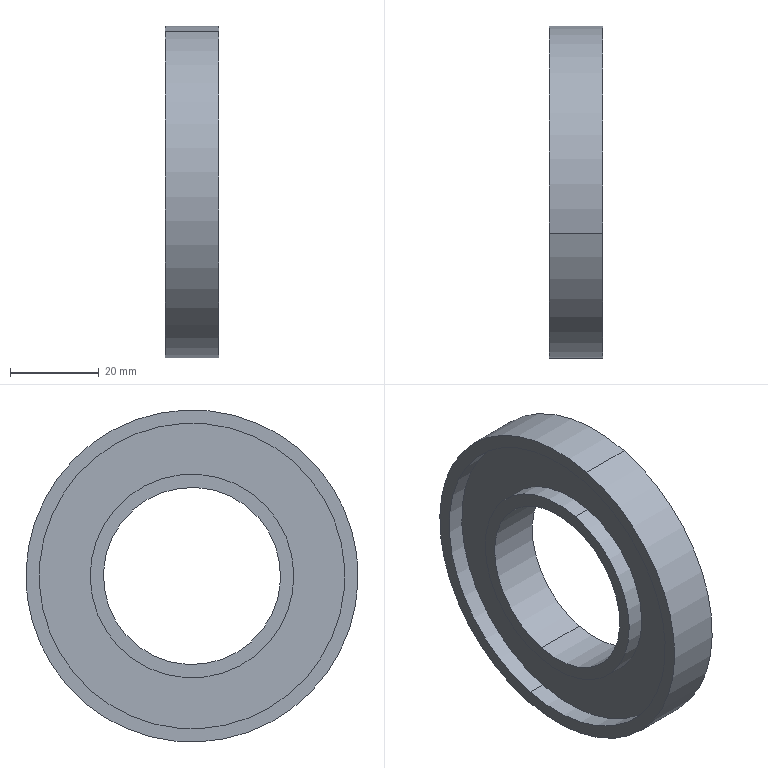Part | NX | features BREP 1 | 1 solid | 18 faces | box 12 x 75 x 75 mm | volume 21316 mm3 | cylinder 12 | plane 6 | commonest cylinder face diameters 46 x4 69 x4 40 x2 75 x2
STEP:
#1=CARTESIAN_POINT('',(691.455,5.743,-22.271));
#2=VERTEX_POINT('',#1);
#3=CARTESIAN_POINT('',(691.455,-5.743,22.271));
#4=VERTEX_POINT('',#3);
#5=CARTESIAN_POINT('',(691.455,0.,0.));
#6=DIRECTION('',(-1.,0.,0.));
#7=DIRECTION('',(0.,-0.2497,0.9683));
#8=AXIS2_PLACEMENT_3D('',#5,#6,#7);
#9=CIRCLE('',#8,23.);
#10=EDGE_CURVE('',#2,#4,#9,.T.);
#11=ORIENTED_EDGE('',*,*,#10,.T.);
#12=CARTESIAN_POINT('',(687.455,-5.743,22.271));
#13=VERTEX_POINT('',#12);
#14=CARTESIAN_POINT('',(691.686,-5.743,22.271));
#15=DIRECTION('',(-1.,0.,0.));
#16=VECTOR('',#15,1000.);
#17=LINE('',#14,#16);
#18=EDGE_CURVE('',#4,#13,#17,.T.);
#19=ORIENTED_EDGE('',*,*,#18,.T.);
#20=CARTESIAN_POINT('',(687.455,5.743,-22.271));
#21=VERTEX_POINT('',#20);
#22=CARTESIAN_POINT('',(687.455,0.,0.));
#23=DIRECTION('',(-1.,0.,0.));
#24=DIRECTION('',(0.,-0.2497,0.9683));
#25=AXIS2_PLACEMENT_3D('',#22,#23,#24);
#26=CIRCLE('',#25,23.);
#27=EDGE_CURVE('',#21,#13,#26,.T.);
#28=ORIENTED_EDGE('',*,*,#27,.F.);
#29=CARTESIAN_POINT('',(691.686,5.743,-22.271));
#30=DIRECTION('',(-1.,0.,0.));
#31=VECTOR('',#30,1000.);
#32=LINE('',#29,#31);
#33=EDGE_CURVE('',#2,#21,#32,.T.);
#34=ORIENTED_EDGE('',*,*,#33,.F.);
#35=EDGE_LOOP('',(#11,#19,#28,#34));
#36=FACE_BOUND('',#35,.T.);
#37=CARTESIAN_POINT('',(691.686,0.,0.));
#38=DIRECTION('',(-1.,0.,0.));
#39=DIRECTION('',(0.,-0.2497,0.9683));
#40=AXIS2_PLACEMENT_3D('',#37,#38,#39);
#41=CYLINDRICAL_SURFACE('',#40,23.);
#42=ADVANCED_FACE('',(#36),#41,.T.);
#43=CARTESIAN_POINT('',(691.455,-8.615,33.407));
#44=VERTEX_POINT('',#43);
#45=CARTESIAN_POINT('',(691.455,8.615,-33.407));
#46=VERTEX_POINT('',#45);
#47=CARTESIAN_POINT('',(691.455,0.,0.));
#48=DIRECTION('',(-1.,0.,0.));
#49=DIRECTION('',(0.,-0.2497,0.9683));
#50=AXIS2_PLACEMENT_3D('',#47,#48,#49);
#51=CIRCLE('',#50,34.5);
#52=EDGE_CURVE('',#44,#46,#51,.T.);
#53=ORIENTED_EDGE('',*,*,#52,.F.);
#54=CARTESIAN_POINT('',(687.455,-8.615,33.407));
#55=VERTEX_POINT('',#54);
#56=CARTESIAN_POINT('',(691.686,-8.615,33.407));
#57=DIRECTION('',(-1.,0.,0.));
#58=VECTOR('',#57,1000.);
#59=LINE('',#56,#58);
#60=EDGE_CURVE('',#44,#55,#59,.T.);
#61=ORIENTED_EDGE('',*,*,#60,.T.);
#62=CARTESIAN_POINT('',(687.455,8.615,-33.407));
#63=VERTEX_POINT('',#62);
#64=CARTESIAN_POINT('',(687.455,0.,0.));
#65=DIRECTION('',(-1.,0.,0.));
#66=DIRECTION('',(0.,-0.2497,0.9683));
#67=AXIS2_PLACEMENT_3D('',#64,#65,#66);
#68=CIRCLE('',#67,34.5);
#69=EDGE_CURVE('',#55,#63,#68,.T.);
#70=ORIENTED_EDGE('',*,*,#69,.T.);
#71=CARTESIAN_POINT('',(691.686,8.615,-33.407));
#72=DIRECTION('',(-1.,0.,0.));
#73=VECTOR('',#72,1000.);
#74=LINE('',#71,#73);
#75=EDGE_CURVE('',#46,#63,#74,.T.);
#76=ORIENTED_EDGE('',*,*,#75,.F.);
#77=EDGE_LOOP('',(#53,#61,#70,#76));
#78=FACE_BOUND('',#77,.T.);
#79=CARTESIAN_POINT('',(691.686,0.,0.));
#80=DIRECTION('',(-1.,0.,0.));
#81=DIRECTION('',(0.,-0.2497,0.9683));
#82=AXIS2_PLACEMENT_3D('',#79,#80,#81);
#83=CYLINDRICAL_SURFACE('',#82,34.5);
#84=ADVANCED_FACE('',(#78),#83,.F.);
#85=CARTESIAN_POINT('',(699.455,9.364,-36.312));
#86=VERTEX_POINT('',#85);
#87=CARTESIAN_POINT('',(699.455,-9.364,36.312));
#88=VERTEX_POINT('',#87);
#89=CARTESIAN_POINT('',(699.455,0.,0.));
#90=DIRECTION('',(-1.,0.,0.));
#91=DIRECTION('',(0.,-0.2497,0.9683));
#92=AXIS2_PLACEMENT_3D('',#89,#90,#91);
#93=CIRCLE('',#92,37.5);
#94=EDGE_CURVE('',#86,#88,#93,.T.);
#95=ORIENTED_EDGE('',*,*,#94,.T.);
#96=CARTESIAN_POINT('',(687.455,-9.364,36.312));
#97=VERTEX_POINT('',#96);
#98=CARTESIAN_POINT('',(691.686,-9.364,36.312));
#99=DIRECTION('',(-1.,0.,0.));
#100=VECTOR('',#99,1000.);
#101=LINE('',#98,#100);
#102=EDGE_CURVE('',#88,#97,#101,.T.);
#103=ORIENTED_EDGE('',*,*,#102,.T.);
#104=CARTESIAN_POINT('',(687.455,9.364,-36.312));
#105=VERTEX_POINT('',#104);
#106=CARTESIAN_POINT('',(687.455,0.,0.));
#107=DIRECTION('',(-1.,0.,0.));
#108=DIRECTION('',(0.,-0.2497,0.9683));
#109=AXIS2_PLACEMENT_3D('',#106,#107,#108);
#110=CIRCLE('',#109,37.5);
#111=EDGE_CURVE('',#105,#97,#110,.T.);
#112=ORIENTED_EDGE('',*,*,#111,.F.);
#113=CARTESIAN_POINT('',(691.686,9.364,-36.312));
#114=DIRECTION('',(-1.,0.,0.));
#115=VECTOR('',#114,1000.);
#116=LINE('',#113,#115);
#117=EDGE_CURVE('',#86,#105,#116,.T.);
#118=ORIENTED_EDGE('',*,*,#117,.F.);
#119=EDGE_LOOP('',(#95,#103,#112,#118));
#120=FACE_BOUND('',#119,.T.);
#121=CARTESIAN_POINT('',(691.686,0.,0.));
#122=DIRECTION('',(-1.,0.,0.));
#123=DIRECTION('',(0.,-0.2497,0.9683));
#124=AXIS2_PLACEMENT_3D('',#121,#122,#123);
#125=CYLINDRICAL_SURFACE('',#124,37.5);
#126=ADVANCED_FACE('',(#120),#125,.T.);
#127=CARTESIAN_POINT('',(699.455,-8.615,33.407));
#128=VERTEX_POINT('',#127);
#129=CARTESIAN_POINT('',(699.455,8.615,-33.407));
#130=VERTEX_POINT('',#129);
#131=CARTESIAN_POINT('',(699.455,0.,0.));
#132=DIRECTION('',(-1.,0.,0.));
#133=DIRECTION('',(0.,-0.2497,0.9683));
#134=AXIS2_PLACEMENT_3D('',#131,#132,#133);
#135=CIRCLE('',#134,34.5);
#136=EDGE_CURVE('',#128,#130,#135,.T.);
#137=ORIENTED_EDGE('',*,*,#136,.F.);
#138=CARTESIAN_POINT('',(695.455,-8.615,33.407));
#139=VERTEX_POINT('',#138);
#140=CARTESIAN_POINT('',(691.686,-8.615,33.407));
#141=DIRECTION('',(-1.,0.,0.));
#142=VECTOR('',#141,1000.);
#143=LINE('',#140,#142);
#144=EDGE_CURVE('',#128,#139,#143,.T.);
#145=ORIENTED_EDGE('',*,*,#144,.T.);
#146=CARTESIAN_POINT('',(695.455,8.615,-33.407));
#147=VERTEX_POINT('',#146);
#148=CARTESIAN_POINT('',(695.455,0.,0.));
#149=DIRECTION('',(-1.,0.,0.));
#150=DIRECTION('',(0.,-0.2497,0.9683));
#151=AXIS2_PLACEMENT_3D('',#148,#149,#150);
#152=CIRCLE('',#151,34.5);
#153=EDGE_CURVE('',#139,#147,#152,.T.);
#154=ORIENTED_EDGE('',*,*,#153,.T.);
#155=CARTESIAN_POINT('',(691.686,8.615,-33.407));
#156=DIRECTION('',(-1.,0.,0.));
#157=VECTOR('',#156,1000.);
#158=LINE('',#155,#157);
#159=EDGE_CURVE('',#130,#147,#158,.T.);
#160=ORIENTED_EDGE('',*,*,#159,.F.);
#161=EDGE_LOOP('',(#137,#145,#154,#160));
#162=FACE_BOUND('',#161,.T.);
#163=CARTESIAN_POINT('',(691.686,0.,0.));
#164=DIRECTION('',(-1.,0.,0.));
#165=DIRECTION('',(0.,-0.2497,0.9683));
#166=AXIS2_PLACEMENT_3D('',#163,#164,#165);
#167=CYLINDRICAL_SURFACE('',#166,34.5);
#168=ADVANCED_FACE('',(#162),#167,.F.);
#169=CARTESIAN_POINT('',(699.455,5.743,-22.271));
#170=VERTEX_POINT('',#169);
#171=CARTESIAN_POINT('',(699.455,-5.743,22.271));
#172=VERTEX_POINT('',#171);
#173=CARTESIAN_POINT('',(699.455,0.,0.));
#174=DIRECTION('',(-1.,0.,0.));
#175=DIRECTION('',(0.,-0.2497,0.9683));
#176=AXIS2_PLACEMENT_3D('',#173,#174,#175);
#177=CIRCLE('',#176,23.);
#178=EDGE_CURVE('',#170,#172,#177,.T.);
#179=ORIENTED_EDGE('',*,*,#178,.T.);
#180=CARTESIAN_POINT('',(695.455,-5.743,22.271));
#181=VERTEX_POINT('',#180);
#182=CARTESIAN_POINT('',(691.686,-5.743,22.271));
#183=DIRECTION('',(-1.,0.,0.));
#184=VECTOR('',#183,1000.);
#185=LINE('',#182,#184);
#186=EDGE_CURVE('',#172,#181,#185,.T.);
#187=ORIENTED_EDGE('',*,*,#186,.T.);
#188=CARTESIAN_POINT('',(695.455,5.743,-22.271));
#189=VERTEX_POINT('',#188);
#190=CARTESIAN_POINT('',(695.455,0.,0.));
#191=DIRECTION('',(-1.,0.,0.));
#192=DIRECTION('',(0.,-0.2497,0.9683));
#193=AXIS2_PLACEMENT_3D('',#190,#191,#192);
#194=CIRCLE('',#193,23.);
#195=EDGE_CURVE('',#189,#181,#194,.T.);
#196=ORIENTED_EDGE('',*,*,#195,.F.);
#197=CARTESIAN_POINT('',(691.686,5.743,-22.271));
#198=DIRECTION('',(-1.,0.,0.));
#199=VECTOR('',#198,1000.);
#200=LINE('',#197,#199);
#201=EDGE_CURVE('',#170,#189,#200,.T.);
#202=ORIENTED_EDGE('',*,*,#201,.F.);
#203=EDGE_LOOP('',(#179,#187,#196,#202));
#204=FACE_BOUND('',#203,.T.);
#205=CARTESIAN_POINT('',(691.686,0.,0.));
#206=DIRECTION('',(-1.,0.,0.));
#207=DIRECTION('',(0.,-0.2497,0.9683));
#208=AXIS2_PLACEMENT_3D('',#205,#206,#207);
#209=CYLINDRICAL_SURFACE('',#208,23.);
#210=ADVANCED_FACE('',(#204),#209,.T.);
#211=CARTESIAN_POINT('',(699.455,-4.994,19.366));
#212=VERTEX_POINT('',#211);
#213=CARTESIAN_POINT('',(699.455,4.994,-19.366));
#214=VERTEX_POINT('',#213);
#215=CARTESIAN_POINT('',(699.455,0.,0.));
#216=DIRECTION('',(-1.,0.,0.));
#217=DIRECTION('',(0.,-0.2497,0.9683));
#218=AXIS2_PLACEMENT_3D('',#215,#216,#217);
#219=CIRCLE('',#218,20.);
#220=EDGE_CURVE('',#212,#214,#219,.T.);
#221=ORIENTED_EDGE('',*,*,#220,.F.);
#222=CARTESIAN_POINT('',(687.455,-4.994,19.366));
#223=VERTEX_POINT('',#222);
#224=CARTESIAN_POINT('',(691.686,-4.994,19.366));
#225=DIRECTION('',(-1.,0.,0.));
#226=VECTOR('',#225,1000.);
#227=LINE('',#224,#226);
#228=EDGE_CURVE('',#212,#223,#227,.T.);
#229=ORIENTED_EDGE('',*,*,#228,.T.);
#230=CARTESIAN_POINT('',(687.455,4.994,-19.366));
#231=VERTEX_POINT('',#230);
#232=CARTESIAN_POINT('',(687.455,0.,0.));
#233=DIRECTION('',(-1.,0.,0.));
#234=DIRECTION('',(0.,-0.2497,0.9683));
#235=AXIS2_PLACEMENT_3D('',#232,#233,#234);
#236=CIRCLE('',#235,20.);
#237=EDGE_CURVE('',#223,#231,#236,.T.);
#238=ORIENTED_EDGE('',*,*,#237,.T.);
#239=CARTESIAN_POINT('',(691.686,4.994,-19.366));
#240=DIRECTION('',(-1.,0.,0.));
#241=VECTOR('',#240,1000.);
#242=LINE('',#239,#241);
#243=EDGE_CURVE('',#214,#231,#242,.T.);
#244=ORIENTED_EDGE('',*,*,#243,.F.);
#245=EDGE_LOOP('',(#221,#229,#238,#244));
#246=FACE_BOUND('',#245,.T.);
#247=CARTESIAN_POINT('',(691.686,0.,0.));
#248=DIRECTION('',(-1.,0.,0.));
#249=DIRECTION('',(0.,-0.2497,0.9683));
#250=AXIS2_PLACEMENT_3D('',#247,#248,#249);
#251=CYLINDRICAL_SURFACE('',#250,20.);
#252=ADVANCED_FACE('',(#246),#251,.F.);
#253=ORIENTED_EDGE('',*,*,#243,.T.);
#254=CARTESIAN_POINT('',(687.455,0.,0.));
#255=DIRECTION('',(-1.,0.,0.));
#256=DIRECTION('',(0.,-0.2497,0.9683));
#257=AXIS2_PLACEMENT_3D('',#254,#255,#256);
#258=CIRCLE('',#257,20.);
#259=EDGE_CURVE('',#231,#223,#258,.T.);
#260=ORIENTED_EDGE('',*,*,#259,.T.);
#261=ORIENTED_EDGE('',*,*,#228,.F.);
#262=CARTESIAN_POINT('',(699.455,0.,0.));
#263=DIRECTION('',(-1.,0.,0.));
#264=DIRECTION('',(0.,-0.2497,0.9683));
#265=AXIS2_PLACEMENT_3D('',#262,#263,#264);
#266=CIRCLE('',#265,20.);
#267=EDGE_CURVE('',#214,#212,#266,.T.);
#268=ORIENTED_EDGE('',*,*,#267,.F.);
#269=EDGE_LOOP('',(#253,#260,#261,#268));
#270=FACE_BOUND('',#269,.T.);
#271=CARTESIAN_POINT('',(691.686,0.,0.));
#272=DIRECTION('',(-1.,0.,0.));
#273=DIRECTION('',(0.,-0.2497,0.9683));
#274=AXIS2_PLACEMENT_3D('',#271,#272,#273);
#275=CYLINDRICAL_SURFACE('',#274,20.);
#276=ADVANCED_FACE('',(#270),#275,.F.);
#277=ORIENTED_EDGE('',*,*,#178,.F.);
#278=CARTESIAN_POINT('',(699.455,0.,0.));
#279=DIRECTION('',(-1.,0.,0.));
#280=DIRECTION('',(0.,-0.2497,0.9683));
#281=AXIS2_PLACEMENT_3D('',#278,#279,#280);
#282=CIRCLE('',#281,23.);
#283=EDGE_CURVE('',#172,#170,#282,.T.);
#284=ORIENTED_EDGE('',*,*,#283,.F.);
#285=EDGE_LOOP('',(#277,#284));
#286=FACE_BOUND('',#285,.T.);
#287=ORIENTED_EDGE('',*,*,#267,.T.);
#288=ORIENTED_EDGE('',*,*,#220,.T.);
#289=EDGE_LOOP('',(#287,#288));
#290=FACE_BOUND('',#289,.T.);
#291=CARTESIAN_POINT('',(699.455,-19.366,-4.994));
#292=DIRECTION('',(-1.,0.,0.));
#293=DIRECTION('',(0.,-0.2497,0.9683));
#294=AXIS2_PLACEMENT_3D('',#291,#292,#293);
#295=PLANE('',#294);
#296=ADVANCED_FACE('',(#286,#290),#295,.F.);
#297=ORIENTED_EDGE('',*,*,#201,.T.);
#298=CARTESIAN_POINT('',(695.455,0.,0.));
#299=DIRECTION('',(-1.,0.,0.));
#300=DIRECTION('',(0.,-0.2497,0.9683));
#301=AXIS2_PLACEMENT_3D('',#298,#299,#300);
#302=CIRCLE('',#301,23.);
#303=EDGE_CURVE('',#181,#189,#302,.T.);
#304=ORIENTED_EDGE('',*,*,#303,.F.);
#305=ORIENTED_EDGE('',*,*,#186,.F.);
#306=ORIENTED_EDGE('',*,*,#283,.T.);
#307=EDGE_LOOP('',(#297,#304,#305,#306));
#308=FACE_BOUND('',#307,.T.);
#309=CARTESIAN_POINT('',(691.686,0.,0.));
#310=DIRECTION('',(-1.,0.,0.));
#311=DIRECTION('',(0.,-0.2497,0.9683));
#312=AXIS2_PLACEMENT_3D('',#309,#310,#311);
#313=CYLINDRICAL_SURFACE('',#312,23.);
#314=ADVANCED_FACE('',(#308),#313,.T.);
#315=CARTESIAN_POINT('',(695.455,0.,0.));
#316=DIRECTION('',(-1.,0.,0.));
#317=DIRECTION('',(0.,-0.2497,0.9683));
#318=AXIS2_PLACEMENT_3D('',#315,#316,#317);
#319=CIRCLE('',#318,34.5);
#320=EDGE_CURVE('',#147,#139,#319,.T.);
#321=ORIENTED_EDGE('',*,*,#320,.F.);
#322=ORIENTED_EDGE('',*,*,#153,.F.);
#323=EDGE_LOOP('',(#321,#322));
#324=FACE_BOUND('',#323,.T.);
#325=ORIENTED_EDGE('',*,*,#195,.T.);
#326=ORIENTED_EDGE('',*,*,#303,.T.);
#327=EDGE_LOOP('',(#325,#326));
#328=FACE_BOUND('',#327,.T.);
#329=CARTESIAN_POINT('',(695.455,-22.271,-5.743));
#330=DIRECTION('',(-1.,0.,0.));
#331=DIRECTION('',(0.,-0.2497,0.9683));
#332=AXIS2_PLACEMENT_3D('',#329,#330,#331);
#333=PLANE('',#332);
#334=ADVANCED_FACE('',(#324,#328),#333,.F.);
#335=ORIENTED_EDGE('',*,*,#159,.T.);
#336=ORIENTED_EDGE('',*,*,#320,.T.);
#337=ORIENTED_EDGE('',*,*,#144,.F.);
#338=CARTESIAN_POINT('',(699.455,0.,0.));
#339=DIRECTION('',(-1.,0.,0.));
#340=DIRECTION('',(0.,-0.2497,0.9683));
#341=AXIS2_PLACEMENT_3D('',#338,#339,#340);
#342=CIRCLE('',#341,34.5);
#343=EDGE_CURVE('',#130,#128,#342,.T.);
#344=ORIENTED_EDGE('',*,*,#343,.F.);
#345=EDGE_LOOP('',(#335,#336,#337,#344));
#346=FACE_BOUND('',#345,.T.);
#347=CARTESIAN_POINT('',(691.686,0.,0.));
#348=DIRECTION('',(-1.,0.,0.));
#349=DIRECTION('',(0.,-0.2497,0.9683));
#350=AXIS2_PLACEMENT_3D('',#347,#348,#349);
#351=CYLINDRICAL_SURFACE('',#350,34.5);
#352=ADVANCED_FACE('',(#346),#351,.F.);
#353=ORIENTED_EDGE('',*,*,#94,.F.);
#354=CARTESIAN_POINT('',(699.455,0.,0.));
#355=DIRECTION('',(-1.,0.,0.));
#356=DIRECTION('',(0.,-0.2497,0.9683));
#357=AXIS2_PLACEMENT_3D('',#354,#355,#356);
#358=CIRCLE('',#357,37.5);
#359=EDGE_CURVE('',#88,#86,#358,.T.);
#360=ORIENTED_EDGE('',*,*,#359,.F.);
#361=EDGE_LOOP('',(#353,#360));
#362=FACE_BOUND('',#361,.T.);
#363=ORIENTED_EDGE('',*,*,#343,.T.);
#364=ORIENTED_EDGE('',*,*,#136,.T.);
#365=EDGE_LOOP('',(#363,#364));
#366=FACE_BOUND('',#365,.T.);
#367=CARTESIAN_POINT('',(699.455,-33.407,-8.615));
#368=DIRECTION('',(-1.,0.,0.));
#369=DIRECTION('',(0.,-0.2497,0.9683));
#370=AXIS2_PLACEMENT_3D('',#367,#368,#369);
#371=PLANE('',#370);
#372=ADVANCED_FACE('',(#362,#366),#371,.F.);
#373=ORIENTED_EDGE('',*,*,#117,.T.);
#374=CARTESIAN_POINT('',(687.455,0.,0.));
#375=DIRECTION('',(-1.,0.,0.));
#376=DIRECTION('',(0.,-0.2497,0.9683));
#377=AXIS2_PLACEMENT_3D('',#374,#375,#376);
#378=CIRCLE('',#377,37.5);
#379=EDGE_CURVE('',#97,#105,#378,.T.);
#380=ORIENTED_EDGE('',*,*,#379,.F.);
#381=ORIENTED_EDGE('',*,*,#102,.F.);
#382=ORIENTED_EDGE('',*,*,#359,.T.);
#383=EDGE_LOOP('',(#373,#380,#381,#382));
#384=FACE_BOUND('',#383,.T.);
#385=CARTESIAN_POINT('',(691.686,0.,0.));
#386=DIRECTION('',(-1.,0.,0.));
#387=DIRECTION('',(0.,-0.2497,0.9683));
#388=AXIS2_PLACEMENT_3D('',#385,#386,#387);
#389=CYLINDRICAL_SURFACE('',#388,37.5);
#390=ADVANCED_FACE('',(#384),#389,.T.);
#391=CARTESIAN_POINT('',(687.455,0.,0.));
#392=DIRECTION('',(-1.,0.,0.));
#393=DIRECTION('',(0.,-0.2497,0.9683));
#394=AXIS2_PLACEMENT_3D('',#391,#392,#393);
#395=CIRCLE('',#394,34.5);
#396=EDGE_CURVE('',#63,#55,#395,.T.);
#397=ORIENTED_EDGE('',*,*,#396,.F.);
#398=ORIENTED_EDGE('',*,*,#69,.F.);
#399=EDGE_LOOP('',(#397,#398));
#400=FACE_BOUND('',#399,.T.);
#401=ORIENTED_EDGE('',*,*,#111,.T.);
#402=ORIENTED_EDGE('',*,*,#379,.T.);
#403=EDGE_LOOP('',(#401,#402));
#404=FACE_BOUND('',#403,.T.);
#405=CARTESIAN_POINT('',(687.455,-36.312,-9.364));
#406=DIRECTION('',(1.,0.,0.));
#407=DIRECTION('',(0.,0.2497,-0.9683));
#408=AXIS2_PLACEMENT_3D('',#405,#406,#407);
#409=PLANE('',#408);
#410=ADVANCED_FACE('',(#400,#404),#409,.F.);
#411=ORIENTED_EDGE('',*,*,#75,.T.);
#412=ORIENTED_EDGE('',*,*,#396,.T.);
#413=ORIENTED_EDGE('',*,*,#60,.F.);
#414=CARTESIAN_POINT('',(691.455,0.,0.));
#415=DIRECTION('',(-1.,0.,0.));
#416=DIRECTION('',(0.,-0.2497,0.9683));
#417=AXIS2_PLACEMENT_3D('',#414,#415,#416);
#418=CIRCLE('',#417,34.5);
#419=EDGE_CURVE('',#46,#44,#418,.T.);
#420=ORIENTED_EDGE('',*,*,#419,.F.);
#421=EDGE_LOOP('',(#411,#412,#413,#420));
#422=FACE_BOUND('',#421,.T.);
#423=CARTESIAN_POINT('',(691.686,0.,0.));
#424=DIRECTION('',(-1.,0.,0.));
#425=DIRECTION('',(0.,-0.2497,0.9683));
#426=AXIS2_PLACEMENT_3D('',#423,#424,#425);
#427=CYLINDRICAL_SURFACE('',#426,34.5);
#428=ADVANCED_FACE('',(#422),#427,.F.);
#429=ORIENTED_EDGE('',*,*,#10,.F.);
#430=CARTESIAN_POINT('',(691.455,0.,0.));
#431=DIRECTION('',(-1.,0.,0.));
#432=DIRECTION('',(0.,-0.2497,0.9683));
#433=AXIS2_PLACEMENT_3D('',#430,#431,#432);
#434=CIRCLE('',#433,23.);
#435=EDGE_CURVE('',#4,#2,#434,.T.);
#436=ORIENTED_EDGE('',*,*,#435,.F.);
#437=EDGE_LOOP('',(#429,#436));
#438=FACE_BOUND('',#437,.T.);
#439=ORIENTED_EDGE('',*,*,#419,.T.);
#440=ORIENTED_EDGE('',*,*,#52,.T.);
#441=EDGE_LOOP('',(#439,#440));
#442=FACE_BOUND('',#441,.T.);
#443=CARTESIAN_POINT('',(691.455,-33.407,-8.615));
#444=DIRECTION('',(1.,0.,0.));
#445=DIRECTION('',(0.,0.2497,-0.9683));
#446=AXIS2_PLACEMENT_3D('',#443,#444,#445);
#447=PLANE('',#446);
#448=ADVANCED_FACE('',(#438,#442),#447,.F.);
#449=ORIENTED_EDGE('',*,*,#33,.T.);
#450=CARTESIAN_POINT('',(687.455,0.,0.));
#451=DIRECTION('',(-1.,0.,0.));
#452=DIRECTION('',(0.,-0.2497,0.9683));
#453=AXIS2_PLACEMENT_3D('',#450,#451,#452);
#454=CIRCLE('',#453,23.);
#455=EDGE_CURVE('',#13,#21,#454,.T.);
#456=ORIENTED_EDGE('',*,*,#455,.F.);
#457=ORIENTED_EDGE('',*,*,#18,.F.);
#458=ORIENTED_EDGE('',*,*,#435,.T.);
#459=EDGE_LOOP('',(#449,#456,#457,#458));
#460=FACE_BOUND('',#459,.T.);
#461=CARTESIAN_POINT('',(691.686,0.,0.));
#462=DIRECTION('',(-1.,0.,0.));
#463=DIRECTION('',(0.,-0.2497,0.9683));
#464=AXIS2_PLACEMENT_3D('',#461,#462,#463);
#465=CYLINDRICAL_SURFACE('',#464,23.);
#466=ADVANCED_FACE('',(#460),#465,.T.);
#467=ORIENTED_EDGE('',*,*,#259,.F.);
#468=ORIENTED_EDGE('',*,*,#237,.F.);
#469=EDGE_LOOP('',(#467,#468));
#470=FACE_BOUND('',#469,.T.);
#471=ORIENTED_EDGE('',*,*,#27,.T.);
#472=ORIENTED_EDGE('',*,*,#455,.T.);
#473=EDGE_LOOP('',(#471,#472));
#474=FACE_BOUND('',#473,.T.);
#475=CARTESIAN_POINT('',(687.455,-22.271,-5.743));
#476=DIRECTION('',(1.,0.,0.));
#477=DIRECTION('',(0.,0.2497,-0.9683));
#478=AXIS2_PLACEMENT_3D('',#475,#476,#477);
#479=PLANE('',#478);
#480=ADVANCED_FACE('',(#470,#474),#479,.F.);
#481=CLOSED_SHELL('',(#42,#84,#126,#168,#210,#252,#276,#296,#314,#334,#352,#372,#390,#410,#428,#448,#466,#480));
#482=MANIFOLD_SOLID_BREP('',#481);
#483=(LENGTH_UNIT()NAMED_UNIT(*)SI_UNIT(.MILLI.,.METRE.));
#484=UNCERTAINTY_MEASURE_WITH_UNIT(LENGTH_MEASURE(0.00001),#483,'','');
#485=(NAMED_UNIT(*)PLANE_ANGLE_UNIT()SI_UNIT($,.RADIAN.));
#486=(NAMED_UNIT(*)SI_UNIT($,.STERADIAN.)SOLID_ANGLE_UNIT());
#487=(GEOMETRIC_REPRESENTATION_CONTEXT(3)GLOBAL_UNCERTAINTY_ASSIGNED_CONTEXT((#484))GLOBAL_UNIT_ASSIGNED_CONTEXT((#483,#485,#486))REPRESENTATION_CONTEXT('',''));
#488=ADVANCED_BREP_SHAPE_REPRESENTATION('',(#482),#487);